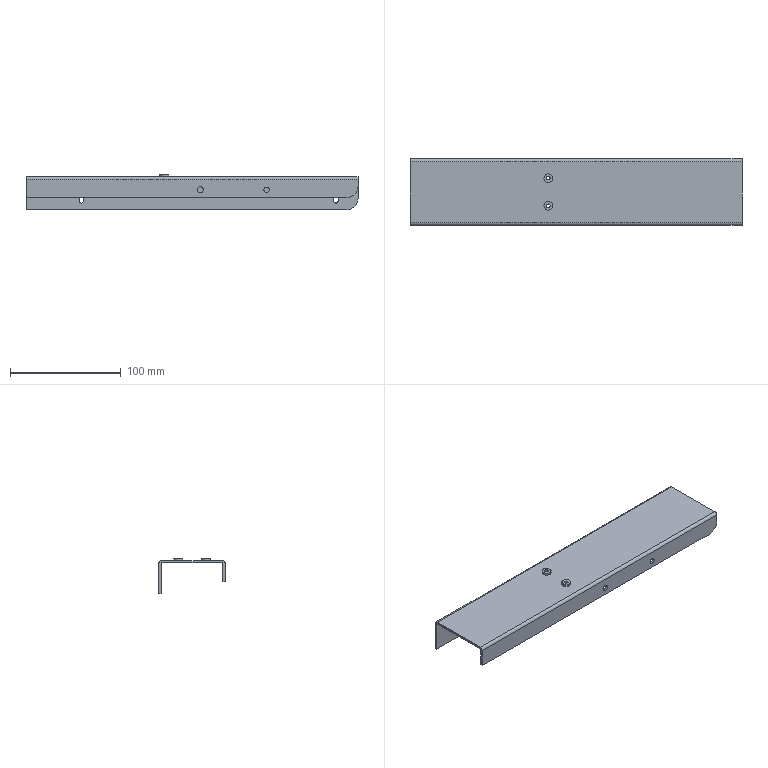Part | STEP file | 1 solid | 32 faces | box 300 x 60 x 32 mm | volume 62070 mm3 | plane 16 | cylinder 16 | commonest cylinder face diameters 4 x4 5 x3 1 x2 3.3 x2 7.9 x2 20 x2